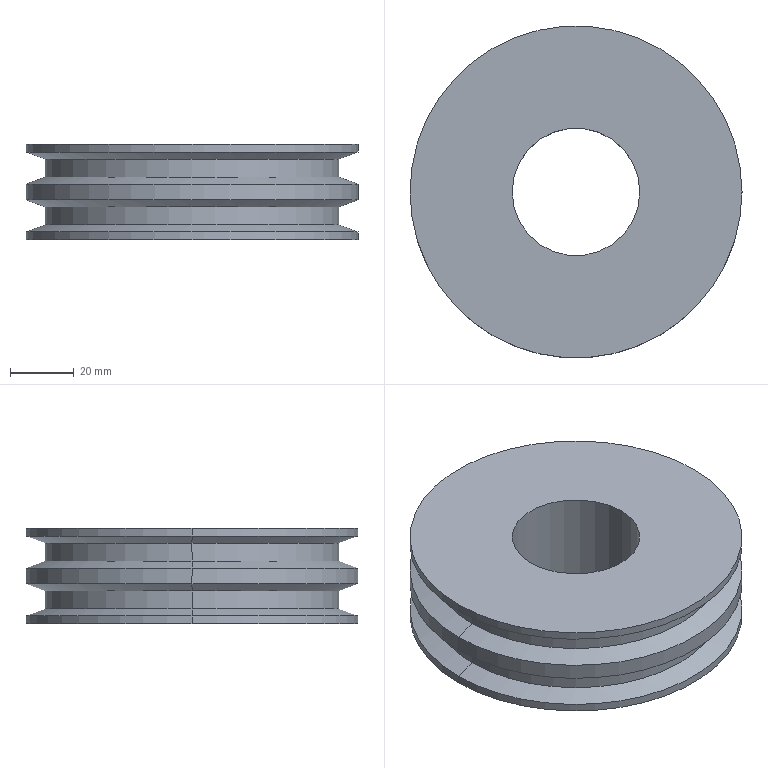Part | SolidWorks | features Extrusion 1, RevCut 1 | 1 solid | 22 faces | box 104 x 104 x 30 mm | volume 188105 mm3 | cylinder 12 | cone 8 | plane 2 | commonest cylinder face diameters 104 x6 92 x4 40 x2
STEP:
#1=CARTESIAN_POINT('',(-52.,0.,17.5));
#2=VERTEX_POINT('',#1);
#3=CARTESIAN_POINT('',(52.,0.,17.5));
#4=VERTEX_POINT('',#3);
#5=CARTESIAN_POINT('',(0.,0.,17.5));
#6=DIRECTION('',(0.,0.,-1.));
#7=DIRECTION('',(-1.,0.,0.));
#8=AXIS2_PLACEMENT_3D('',#5,#6,#7);
#9=CIRCLE('',#8,52.);
#10=EDGE_CURVE('',#2,#4,#9,.T.);
#11=ORIENTED_EDGE('',*,*,#10,.T.);
#12=CARTESIAN_POINT('',(52.,0.,12.5));
#13=VERTEX_POINT('',#12);
#14=CARTESIAN_POINT('',(52.,0.,30.));
#15=DIRECTION('',(0.,0.,-1.));
#16=VECTOR('',#15,1000.);
#17=LINE('',#14,#16);
#18=EDGE_CURVE('',#4,#13,#17,.T.);
#19=ORIENTED_EDGE('',*,*,#18,.T.);
#20=CARTESIAN_POINT('',(-52.,0.,12.5));
#21=VERTEX_POINT('',#20);
#22=CARTESIAN_POINT('',(0.,0.,12.5));
#23=DIRECTION('',(0.,0.,-1.));
#24=DIRECTION('',(-1.,0.,0.));
#25=AXIS2_PLACEMENT_3D('',#22,#23,#24);
#26=CIRCLE('',#25,52.);
#27=EDGE_CURVE('',#21,#13,#26,.T.);
#28=ORIENTED_EDGE('',*,*,#27,.F.);
#29=CARTESIAN_POINT('',(-52.,0.,30.));
#30=DIRECTION('',(0.,0.,-1.));
#31=VECTOR('',#30,1000.);
#32=LINE('',#29,#31);
#33=EDGE_CURVE('',#2,#21,#32,.T.);
#34=ORIENTED_EDGE('',*,*,#33,.F.);
#35=EDGE_LOOP('',(#11,#19,#28,#34));
#36=FACE_OUTER_BOUND('',#35,.T.);
#37=CARTESIAN_POINT('',(0.,0.,30.));
#38=DIRECTION('',(0.,0.,-1.));
#39=DIRECTION('',(-1.,0.,0.));
#40=AXIS2_PLACEMENT_3D('',#37,#38,#39);
#41=CYLINDRICAL_SURFACE('',#40,52.);
#42=ADVANCED_FACE('',(#36),#41,.T.);
#43=CARTESIAN_POINT('',(-46.,0.,19.684));
#44=VERTEX_POINT('',#43);
#45=CARTESIAN_POINT('',(46.,0.,19.684));
#46=VERTEX_POINT('',#45);
#47=CARTESIAN_POINT('',(0.,0.,19.684));
#48=DIRECTION('',(0.,0.,-1.));
#49=DIRECTION('',(-1.,0.,0.));
#50=AXIS2_PLACEMENT_3D('',#47,#48,#49);
#51=CIRCLE('',#50,46.);
#52=EDGE_CURVE('',#44,#46,#51,.T.);
#53=ORIENTED_EDGE('',*,*,#52,.T.);
#54=CARTESIAN_POINT('',(46.,0.,19.684));
#55=DIRECTION('',(0.9397,0.,-0.342));
#56=VECTOR('',#55,1000.);
#57=LINE('',#54,#56);
#58=EDGE_CURVE('',#46,#4,#57,.T.);
#59=ORIENTED_EDGE('',*,*,#58,.T.);
#60=ORIENTED_EDGE('',*,*,#10,.F.);
#61=CARTESIAN_POINT('',(-46.,0.,19.684));
#62=DIRECTION('',(-0.9397,0.,-0.342));
#63=VECTOR('',#62,1000.);
#64=LINE('',#61,#63);
#65=EDGE_CURVE('',#44,#2,#64,.T.);
#66=ORIENTED_EDGE('',*,*,#65,.F.);
#67=EDGE_LOOP('',(#53,#59,#60,#66));
#68=FACE_OUTER_BOUND('',#67,.T.);
#69=CARTESIAN_POINT('',(0.,0.,19.684));
#70=DIRECTION('',(0.,0.,-1.));
#71=DIRECTION('',(-1.,0.,0.));
#72=AXIS2_PLACEMENT_3D('',#69,#70,#71);
#73=CONICAL_SURFACE('',#72,46.,1.222);
#74=ADVANCED_FACE('',(#68),#73,.T.);
#75=CARTESIAN_POINT('',(-46.,0.,25.316));
#76=VERTEX_POINT('',#75);
#77=CARTESIAN_POINT('',(46.,0.,25.316));
#78=VERTEX_POINT('',#77);
#79=CARTESIAN_POINT('',(0.,0.,25.316));
#80=DIRECTION('',(0.,0.,-1.));
#81=DIRECTION('',(-1.,0.,0.));
#82=AXIS2_PLACEMENT_3D('',#79,#80,#81);
#83=CIRCLE('',#82,46.);
#84=EDGE_CURVE('',#76,#78,#83,.T.);
#85=ORIENTED_EDGE('',*,*,#84,.T.);
#86=CARTESIAN_POINT('',(46.,0.,0.));
#87=DIRECTION('',(0.,0.,-1.));
#88=VECTOR('',#87,1000.);
#89=LINE('',#86,#88);
#90=EDGE_CURVE('',#78,#46,#89,.T.);
#91=ORIENTED_EDGE('',*,*,#90,.T.);
#92=ORIENTED_EDGE('',*,*,#52,.F.);
#93=CARTESIAN_POINT('',(-46.,0.,0.));
#94=DIRECTION('',(0.,0.,-1.));
#95=VECTOR('',#94,1000.);
#96=LINE('',#93,#95);
#97=EDGE_CURVE('',#76,#44,#96,.T.);
#98=ORIENTED_EDGE('',*,*,#97,.F.);
#99=EDGE_LOOP('',(#85,#91,#92,#98));
#100=FACE_OUTER_BOUND('',#99,.T.);
#101=CARTESIAN_POINT('',(0.,0.,0.));
#102=DIRECTION('',(0.,0.,-1.));
#103=DIRECTION('',(-1.,0.,0.));
#104=AXIS2_PLACEMENT_3D('',#101,#102,#103);
#105=CYLINDRICAL_SURFACE('',#104,46.);
#106=ADVANCED_FACE('',(#100),#105,.T.);
#107=ORIENTED_EDGE('',*,*,#84,.F.);
#108=CARTESIAN_POINT('',(-52.,0.,27.5));
#109=VERTEX_POINT('',#108);
#110=CARTESIAN_POINT('',(-52.,0.,27.5));
#111=DIRECTION('',(-0.9397,0.,0.342));
#112=VECTOR('',#111,1000.);
#113=LINE('',#110,#112);
#114=EDGE_CURVE('',#76,#109,#113,.T.);
#115=ORIENTED_EDGE('',*,*,#114,.T.);
#116=CARTESIAN_POINT('',(52.,0.,27.5));
#117=VERTEX_POINT('',#116);
#118=CARTESIAN_POINT('',(0.,0.,27.5));
#119=DIRECTION('',(0.,0.,-1.));
#120=DIRECTION('',(-1.,0.,0.));
#121=AXIS2_PLACEMENT_3D('',#118,#119,#120);
#122=CIRCLE('',#121,52.);
#123=EDGE_CURVE('',#109,#117,#122,.T.);
#124=ORIENTED_EDGE('',*,*,#123,.T.);
#125=CARTESIAN_POINT('',(52.,0.,27.5));
#126=DIRECTION('',(0.9397,0.,0.342));
#127=VECTOR('',#126,1000.);
#128=LINE('',#125,#127);
#129=EDGE_CURVE('',#78,#117,#128,.T.);
#130=ORIENTED_EDGE('',*,*,#129,.F.);
#131=EDGE_LOOP('',(#107,#115,#124,#130));
#132=FACE_OUTER_BOUND('',#131,.T.);
#133=CARTESIAN_POINT('',(0.,0.,27.5));
#134=DIRECTION('',(0.,0.,1.));
#135=DIRECTION('',(1.,0.,0.));
#136=AXIS2_PLACEMENT_3D('',#133,#134,#135);
#137=CONICAL_SURFACE('',#136,52.,1.222);
#138=ADVANCED_FACE('',(#132),#137,.T.);
#139=CARTESIAN_POINT('',(-46.,0.,10.316));
#140=VERTEX_POINT('',#139);
#141=CARTESIAN_POINT('',(46.,0.,10.316));
#142=VERTEX_POINT('',#141);
#143=CARTESIAN_POINT('',(0.,0.,10.316));
#144=DIRECTION('',(0.,0.,-1.));
#145=DIRECTION('',(-1.,0.,0.));
#146=AXIS2_PLACEMENT_3D('',#143,#144,#145);
#147=CIRCLE('',#146,46.);
#148=EDGE_CURVE('',#140,#142,#147,.T.);
#149=ORIENTED_EDGE('',*,*,#148,.F.);
#150=CARTESIAN_POINT('',(-52.,0.,12.5));
#151=DIRECTION('',(-0.9397,0.,0.342));
#152=VECTOR('',#151,1000.);
#153=LINE('',#150,#152);
#154=EDGE_CURVE('',#140,#21,#153,.T.);
#155=ORIENTED_EDGE('',*,*,#154,.T.);
#156=ORIENTED_EDGE('',*,*,#27,.T.);
#157=CARTESIAN_POINT('',(52.,0.,12.5));
#158=DIRECTION('',(0.9397,0.,0.342));
#159=VECTOR('',#158,1000.);
#160=LINE('',#157,#159);
#161=EDGE_CURVE('',#142,#13,#160,.T.);
#162=ORIENTED_EDGE('',*,*,#161,.F.);
#163=EDGE_LOOP('',(#149,#155,#156,#162));
#164=FACE_OUTER_BOUND('',#163,.T.);
#165=CARTESIAN_POINT('',(0.,0.,12.5));
#166=DIRECTION('',(0.,0.,1.));
#167=DIRECTION('',(1.,0.,0.));
#168=AXIS2_PLACEMENT_3D('',#165,#166,#167);
#169=CONICAL_SURFACE('',#168,52.,1.222);
#170=ADVANCED_FACE('',(#164),#169,.T.);
#171=ORIENTED_EDGE('',*,*,#148,.T.);
#172=CARTESIAN_POINT('',(46.,0.,4.684));
#173=VERTEX_POINT('',#172);
#174=CARTESIAN_POINT('',(46.,0.,0.));
#175=DIRECTION('',(0.,0.,-1.));
#176=VECTOR('',#175,1000.);
#177=LINE('',#174,#176);
#178=EDGE_CURVE('',#142,#173,#177,.T.);
#179=ORIENTED_EDGE('',*,*,#178,.T.);
#180=CARTESIAN_POINT('',(-46.,0.,4.684));
#181=VERTEX_POINT('',#180);
#182=CARTESIAN_POINT('',(0.,0.,4.684));
#183=DIRECTION('',(0.,0.,-1.));
#184=DIRECTION('',(-1.,0.,0.));
#185=AXIS2_PLACEMENT_3D('',#182,#183,#184);
#186=CIRCLE('',#185,46.);
#187=EDGE_CURVE('',#181,#173,#186,.T.);
#188=ORIENTED_EDGE('',*,*,#187,.F.);
#189=CARTESIAN_POINT('',(-46.,0.,0.));
#190=DIRECTION('',(0.,0.,-1.));
#191=VECTOR('',#190,1000.);
#192=LINE('',#189,#191);
#193=EDGE_CURVE('',#140,#181,#192,.T.);
#194=ORIENTED_EDGE('',*,*,#193,.F.);
#195=EDGE_LOOP('',(#171,#179,#188,#194));
#196=FACE_OUTER_BOUND('',#195,.T.);
#197=CARTESIAN_POINT('',(0.,0.,0.));
#198=DIRECTION('',(0.,0.,-1.));
#199=DIRECTION('',(-1.,0.,0.));
#200=AXIS2_PLACEMENT_3D('',#197,#198,#199);
#201=CYLINDRICAL_SURFACE('',#200,46.);
#202=ADVANCED_FACE('',(#196),#201,.T.);
#203=ORIENTED_EDGE('',*,*,#187,.T.);
#204=CARTESIAN_POINT('',(52.,0.,2.5));
#205=VERTEX_POINT('',#204);
#206=CARTESIAN_POINT('',(46.,0.,4.684));
#207=DIRECTION('',(0.9397,0.,-0.342));
#208=VECTOR('',#207,1000.);
#209=LINE('',#206,#208);
#210=EDGE_CURVE('',#173,#205,#209,.T.);
#211=ORIENTED_EDGE('',*,*,#210,.T.);
#212=CARTESIAN_POINT('',(-52.,0.,2.5));
#213=VERTEX_POINT('',#212);
#214=CARTESIAN_POINT('',(0.,0.,2.5));
#215=DIRECTION('',(0.,0.,-1.));
#216=DIRECTION('',(-1.,0.,0.));
#217=AXIS2_PLACEMENT_3D('',#214,#215,#216);
#218=CIRCLE('',#217,52.);
#219=EDGE_CURVE('',#213,#205,#218,.T.);
#220=ORIENTED_EDGE('',*,*,#219,.F.);
#221=CARTESIAN_POINT('',(-46.,0.,4.684));
#222=DIRECTION('',(-0.9397,0.,-0.342));
#223=VECTOR('',#222,1000.);
#224=LINE('',#221,#223);
#225=EDGE_CURVE('',#181,#213,#224,.T.);
#226=ORIENTED_EDGE('',*,*,#225,.F.);
#227=EDGE_LOOP('',(#203,#211,#220,#226));
#228=FACE_OUTER_BOUND('',#227,.T.);
#229=CARTESIAN_POINT('',(0.,0.,4.684));
#230=DIRECTION('',(0.,0.,-1.));
#231=DIRECTION('',(-1.,0.,0.));
#232=AXIS2_PLACEMENT_3D('',#229,#230,#231);
#233=CONICAL_SURFACE('',#232,46.,1.222);
#234=ADVANCED_FACE('',(#228),#233,.T.);
#235=CARTESIAN_POINT('',(-20.,0.,30.));
#236=VERTEX_POINT('',#235);
#237=CARTESIAN_POINT('',(20.,0.,30.));
#238=VERTEX_POINT('',#237);
#239=CARTESIAN_POINT('',(0.,0.,30.));
#240=DIRECTION('',(0.,0.,1.));
#241=DIRECTION('',(1.,0.,0.));
#242=AXIS2_PLACEMENT_3D('',#239,#240,#241);
#243=CIRCLE('',#242,20.);
#244=EDGE_CURVE('',#236,#238,#243,.T.);
#245=ORIENTED_EDGE('',*,*,#244,.T.);
#246=CARTESIAN_POINT('',(20.,0.,0.));
#247=VERTEX_POINT('',#246);
#248=CARTESIAN_POINT('',(20.,0.,30.));
#249=DIRECTION('',(0.,0.,-1.));
#250=VECTOR('',#249,1000.);
#251=LINE('',#248,#250);
#252=EDGE_CURVE('',#238,#247,#251,.T.);
#253=ORIENTED_EDGE('',*,*,#252,.T.);
#254=CARTESIAN_POINT('',(-20.,0.,0.));
#255=VERTEX_POINT('',#254);
#256=CARTESIAN_POINT('',(0.,0.,0.));
#257=DIRECTION('',(0.,0.,1.));
#258=DIRECTION('',(1.,0.,0.));
#259=AXIS2_PLACEMENT_3D('',#256,#257,#258);
#260=CIRCLE('',#259,20.);
#261=EDGE_CURVE('',#255,#247,#260,.T.);
#262=ORIENTED_EDGE('',*,*,#261,.F.);
#263=CARTESIAN_POINT('',(-20.,0.,30.));
#264=DIRECTION('',(0.,0.,-1.));
#265=VECTOR('',#264,1000.);
#266=LINE('',#263,#265);
#267=EDGE_CURVE('',#236,#255,#266,.T.);
#268=ORIENTED_EDGE('',*,*,#267,.F.);
#269=EDGE_LOOP('',(#245,#253,#262,#268));
#270=FACE_OUTER_BOUND('',#269,.T.);
#271=CARTESIAN_POINT('',(0.,0.,30.));
#272=DIRECTION('',(0.,0.,-1.));
#273=DIRECTION('',(-1.,0.,0.));
#274=AXIS2_PLACEMENT_3D('',#271,#272,#273);
#275=CYLINDRICAL_SURFACE('',#274,20.);
#276=ADVANCED_FACE('',(#270),#275,.F.);
#277=ORIENTED_EDGE('',*,*,#219,.T.);
#278=CARTESIAN_POINT('',(52.,0.,0.));
#279=VERTEX_POINT('',#278);
#280=CARTESIAN_POINT('',(52.,0.,30.));
#281=DIRECTION('',(0.,0.,-1.));
#282=VECTOR('',#281,1000.);
#283=LINE('',#280,#282);
#284=EDGE_CURVE('',#205,#279,#283,.T.);
#285=ORIENTED_EDGE('',*,*,#284,.T.);
#286=CARTESIAN_POINT('',(-52.,0.,0.));
#287=VERTEX_POINT('',#286);
#288=CARTESIAN_POINT('',(0.,0.,0.));
#289=DIRECTION('',(0.,0.,1.));
#290=DIRECTION('',(1.,0.,0.));
#291=AXIS2_PLACEMENT_3D('',#288,#289,#290);
#292=CIRCLE('',#291,52.);
#293=EDGE_CURVE('',#279,#287,#292,.T.);
#294=ORIENTED_EDGE('',*,*,#293,.T.);
#295=CARTESIAN_POINT('',(-52.,0.,30.));
#296=DIRECTION('',(0.,0.,-1.));
#297=VECTOR('',#296,1000.);
#298=LINE('',#295,#297);
#299=EDGE_CURVE('',#213,#287,#298,.T.);
#300=ORIENTED_EDGE('',*,*,#299,.F.);
#301=EDGE_LOOP('',(#277,#285,#294,#300));
#302=FACE_OUTER_BOUND('',#301,.T.);
#303=CARTESIAN_POINT('',(0.,0.,30.));
#304=DIRECTION('',(0.,0.,-1.));
#305=DIRECTION('',(-1.,0.,0.));
#306=AXIS2_PLACEMENT_3D('',#303,#304,#305);
#307=CYLINDRICAL_SURFACE('',#306,52.);
#308=ADVANCED_FACE('',(#302),#307,.T.);
#309=CARTESIAN_POINT('',(52.,0.,30.));
#310=VERTEX_POINT('',#309);
#311=CARTESIAN_POINT('',(-52.,0.,30.));
#312=VERTEX_POINT('',#311);
#313=CARTESIAN_POINT('',(0.,0.,30.));
#314=DIRECTION('',(0.,0.,1.));
#315=DIRECTION('',(1.,0.,0.));
#316=AXIS2_PLACEMENT_3D('',#313,#314,#315);
#317=CIRCLE('',#316,52.);
#318=EDGE_CURVE('',#310,#312,#317,.T.);
#319=ORIENTED_EDGE('',*,*,#318,.F.);
#320=CARTESIAN_POINT('',(52.,0.,30.));
#321=DIRECTION('',(0.,0.,-1.));
#322=VECTOR('',#321,1000.);
#323=LINE('',#320,#322);
#324=EDGE_CURVE('',#310,#117,#323,.T.);
#325=ORIENTED_EDGE('',*,*,#324,.T.);
#326=ORIENTED_EDGE('',*,*,#123,.F.);
#327=CARTESIAN_POINT('',(-52.,0.,30.));
#328=DIRECTION('',(0.,0.,-1.));
#329=VECTOR('',#328,1000.);
#330=LINE('',#327,#329);
#331=EDGE_CURVE('',#312,#109,#330,.T.);
#332=ORIENTED_EDGE('',*,*,#331,.F.);
#333=EDGE_LOOP('',(#319,#325,#326,#332));
#334=FACE_OUTER_BOUND('',#333,.T.);
#335=CARTESIAN_POINT('',(0.,0.,30.));
#336=DIRECTION('',(0.,0.,-1.));
#337=DIRECTION('',(-1.,0.,0.));
#338=AXIS2_PLACEMENT_3D('',#335,#336,#337);
#339=CYLINDRICAL_SURFACE('',#338,52.);
#340=ADVANCED_FACE('',(#334),#339,.T.);
#341=ORIENTED_EDGE('',*,*,#324,.F.);
#342=CARTESIAN_POINT('',(0.,0.,30.));
#343=DIRECTION('',(0.,0.,1.));
#344=DIRECTION('',(1.,0.,0.));
#345=AXIS2_PLACEMENT_3D('',#342,#343,#344);
#346=CIRCLE('',#345,52.);
#347=EDGE_CURVE('',#312,#310,#346,.T.);
#348=ORIENTED_EDGE('',*,*,#347,.F.);
#349=ORIENTED_EDGE('',*,*,#331,.T.);
#350=CARTESIAN_POINT('',(0.,0.,27.5));
#351=DIRECTION('',(0.,0.,-1.));
#352=DIRECTION('',(-1.,0.,0.));
#353=AXIS2_PLACEMENT_3D('',#350,#351,#352);
#354=CIRCLE('',#353,52.);
#355=EDGE_CURVE('',#117,#109,#354,.T.);
#356=ORIENTED_EDGE('',*,*,#355,.F.);
#357=EDGE_LOOP('',(#341,#348,#349,#356));
#358=FACE_OUTER_BOUND('',#357,.T.);
#359=CARTESIAN_POINT('',(0.,0.,30.));
#360=DIRECTION('',(0.,0.,-1.));
#361=DIRECTION('',(-1.,0.,0.));
#362=AXIS2_PLACEMENT_3D('',#359,#360,#361);
#363=CYLINDRICAL_SURFACE('',#362,52.);
#364=ADVANCED_FACE('',(#358),#363,.T.);
#365=ORIENTED_EDGE('',*,*,#284,.F.);
#366=CARTESIAN_POINT('',(0.,0.,2.5));
#367=DIRECTION('',(0.,0.,-1.));
#368=DIRECTION('',(-1.,0.,0.));
#369=AXIS2_PLACEMENT_3D('',#366,#367,#368);
#370=CIRCLE('',#369,52.);
#371=EDGE_CURVE('',#205,#213,#370,.T.);
#372=ORIENTED_EDGE('',*,*,#371,.T.);
#373=ORIENTED_EDGE('',*,*,#299,.T.);
#374=CARTESIAN_POINT('',(0.,0.,0.));
#375=DIRECTION('',(0.,0.,1.));
#376=DIRECTION('',(1.,0.,0.));
#377=AXIS2_PLACEMENT_3D('',#374,#375,#376);
#378=CIRCLE('',#377,52.);
#379=EDGE_CURVE('',#287,#279,#378,.T.);
#380=ORIENTED_EDGE('',*,*,#379,.T.);
#381=EDGE_LOOP('',(#365,#372,#373,#380));
#382=FACE_OUTER_BOUND('',#381,.T.);
#383=CARTESIAN_POINT('',(0.,0.,30.));
#384=DIRECTION('',(0.,0.,-1.));
#385=DIRECTION('',(-1.,0.,0.));
#386=AXIS2_PLACEMENT_3D('',#383,#384,#385);
#387=CYLINDRICAL_SURFACE('',#386,52.);
#388=ADVANCED_FACE('',(#382),#387,.T.);
#389=ORIENTED_EDGE('',*,*,#347,.T.);
#390=ORIENTED_EDGE('',*,*,#318,.T.);
#391=EDGE_LOOP('',(#389,#390));
#392=FACE_OUTER_BOUND('',#391,.T.);
#393=ORIENTED_EDGE('',*,*,#244,.F.);
#394=CARTESIAN_POINT('',(0.,0.,30.));
#395=DIRECTION('',(0.,0.,1.));
#396=DIRECTION('',(1.,0.,0.));
#397=AXIS2_PLACEMENT_3D('',#394,#395,#396);
#398=CIRCLE('',#397,20.);
#399=EDGE_CURVE('',#238,#236,#398,.T.);
#400=ORIENTED_EDGE('',*,*,#399,.F.);
#401=EDGE_LOOP('',(#393,#400));
#402=FACE_BOUND('',#401,.T.);
#403=CARTESIAN_POINT('',(0.,0.,30.));
#404=DIRECTION('',(0.,0.,1.));
#405=DIRECTION('',(1.,0.,0.));
#406=AXIS2_PLACEMENT_3D('',#403,#404,#405);
#407=PLANE('',#406);
#408=ADVANCED_FACE('',(#392,#402),#407,.T.);
#409=ORIENTED_EDGE('',*,*,#379,.F.);
#410=ORIENTED_EDGE('',*,*,#293,.F.);
#411=EDGE_LOOP('',(#409,#410));
#412=FACE_OUTER_BOUND('',#411,.T.);
#413=ORIENTED_EDGE('',*,*,#261,.T.);
#414=CARTESIAN_POINT('',(0.,0.,0.));
#415=DIRECTION('',(0.,0.,1.));
#416=DIRECTION('',(1.,0.,0.));
#417=AXIS2_PLACEMENT_3D('',#414,#415,#416);
#418=CIRCLE('',#417,20.);
#419=EDGE_CURVE('',#247,#255,#418,.T.);
#420=ORIENTED_EDGE('',*,*,#419,.T.);
#421=EDGE_LOOP('',(#413,#420));
#422=FACE_BOUND('',#421,.T.);
#423=CARTESIAN_POINT('',(0.,0.,0.));
#424=DIRECTION('',(0.,0.,1.));
#425=DIRECTION('',(1.,0.,0.));
#426=AXIS2_PLACEMENT_3D('',#423,#424,#425);
#427=PLANE('',#426);
#428=ADVANCED_FACE('',(#412,#422),#427,.F.);
#429=ORIENTED_EDGE('',*,*,#252,.F.);
#430=ORIENTED_EDGE('',*,*,#399,.T.);
#431=ORIENTED_EDGE('',*,*,#267,.T.);
#432=ORIENTED_EDGE('',*,*,#419,.F.);
#433=EDGE_LOOP('',(#429,#430,#431,#432));
#434=FACE_OUTER_BOUND('',#433,.T.);
#435=CARTESIAN_POINT('',(0.,0.,30.));
#436=DIRECTION('',(0.,0.,-1.));
#437=DIRECTION('',(-1.,0.,0.));
#438=AXIS2_PLACEMENT_3D('',#435,#436,#437);
#439=CYLINDRICAL_SURFACE('',#438,20.);
#440=ADVANCED_FACE('',(#434),#439,.F.);
#441=ORIENTED_EDGE('',*,*,#210,.F.);
#442=CARTESIAN_POINT('',(0.,0.,4.684));
#443=DIRECTION('',(0.,0.,-1.));
#444=DIRECTION('',(-1.,0.,0.));
#445=AXIS2_PLACEMENT_3D('',#442,#443,#444);
#446=CIRCLE('',#445,46.);
#447=EDGE_CURVE('',#173,#181,#446,.T.);
#448=ORIENTED_EDGE('',*,*,#447,.T.);
#449=ORIENTED_EDGE('',*,*,#225,.T.);
#450=ORIENTED_EDGE('',*,*,#371,.F.);
#451=EDGE_LOOP('',(#441,#448,#449,#450));
#452=FACE_OUTER_BOUND('',#451,.T.);
#453=CARTESIAN_POINT('',(0.,0.,4.684));
#454=DIRECTION('',(0.,0.,-1.));
#455=DIRECTION('',(-1.,0.,0.));
#456=AXIS2_PLACEMENT_3D('',#453,#454,#455);
#457=CONICAL_SURFACE('',#456,46.,1.222);
#458=ADVANCED_FACE('',(#452),#457,.T.);
#459=ORIENTED_EDGE('',*,*,#178,.F.);
#460=CARTESIAN_POINT('',(0.,0.,10.316));
#461=DIRECTION('',(0.,0.,-1.));
#462=DIRECTION('',(-1.,0.,0.));
#463=AXIS2_PLACEMENT_3D('',#460,#461,#462);
#464=CIRCLE('',#463,46.);
#465=EDGE_CURVE('',#142,#140,#464,.T.);
#466=ORIENTED_EDGE('',*,*,#465,.T.);
#467=ORIENTED_EDGE('',*,*,#193,.T.);
#468=ORIENTED_EDGE('',*,*,#447,.F.);
#469=EDGE_LOOP('',(#459,#466,#467,#468));
#470=FACE_OUTER_BOUND('',#469,.T.);
#471=CARTESIAN_POINT('',(0.,0.,0.));
#472=DIRECTION('',(0.,0.,-1.));
#473=DIRECTION('',(-1.,0.,0.));
#474=AXIS2_PLACEMENT_3D('',#471,#472,#473);
#475=CYLINDRICAL_SURFACE('',#474,46.);
#476=ADVANCED_FACE('',(#470),#475,.T.);
#477=ORIENTED_EDGE('',*,*,#154,.F.);
#478=ORIENTED_EDGE('',*,*,#465,.F.);
#479=ORIENTED_EDGE('',*,*,#161,.T.);
#480=CARTESIAN_POINT('',(0.,0.,12.5));
#481=DIRECTION('',(0.,0.,-1.));
#482=DIRECTION('',(-1.,0.,0.));
#483=AXIS2_PLACEMENT_3D('',#480,#481,#482);
#484=CIRCLE('',#483,52.);
#485=EDGE_CURVE('',#13,#21,#484,.T.);
#486=ORIENTED_EDGE('',*,*,#485,.T.);
#487=EDGE_LOOP('',(#477,#478,#479,#486));
#488=FACE_OUTER_BOUND('',#487,.T.);
#489=CARTESIAN_POINT('',(0.,0.,12.5));
#490=DIRECTION('',(0.,0.,1.));
#491=DIRECTION('',(1.,0.,0.));
#492=AXIS2_PLACEMENT_3D('',#489,#490,#491);
#493=CONICAL_SURFACE('',#492,52.,1.222);
#494=ADVANCED_FACE('',(#488),#493,.T.);
#495=ORIENTED_EDGE('',*,*,#114,.F.);
#496=CARTESIAN_POINT('',(0.,0.,25.316));
#497=DIRECTION('',(0.,0.,-1.));
#498=DIRECTION('',(-1.,0.,0.));
#499=AXIS2_PLACEMENT_3D('',#496,#497,#498);
#500=CIRCLE('',#499,46.);
#501=EDGE_CURVE('',#78,#76,#500,.T.);
#502=ORIENTED_EDGE('',*,*,#501,.F.);
#503=ORIENTED_EDGE('',*,*,#129,.T.);
#504=ORIENTED_EDGE('',*,*,#355,.T.);
#505=EDGE_LOOP('',(#495,#502,#503,#504));
#506=FACE_OUTER_BOUND('',#505,.T.);
#507=CARTESIAN_POINT('',(0.,0.,27.5));
#508=DIRECTION('',(0.,0.,1.));
#509=DIRECTION('',(1.,0.,0.));
#510=AXIS2_PLACEMENT_3D('',#507,#508,#509);
#511=CONICAL_SURFACE('',#510,52.,1.222);
#512=ADVANCED_FACE('',(#506),#511,.T.);
#513=ORIENTED_EDGE('',*,*,#90,.F.);
#514=ORIENTED_EDGE('',*,*,#501,.T.);
#515=ORIENTED_EDGE('',*,*,#97,.T.);
#516=CARTESIAN_POINT('',(0.,0.,19.684));
#517=DIRECTION('',(0.,0.,-1.));
#518=DIRECTION('',(-1.,0.,0.));
#519=AXIS2_PLACEMENT_3D('',#516,#517,#518);
#520=CIRCLE('',#519,46.);
#521=EDGE_CURVE('',#46,#44,#520,.T.);
#522=ORIENTED_EDGE('',*,*,#521,.F.);
#523=EDGE_LOOP('',(#513,#514,#515,#522));
#524=FACE_OUTER_BOUND('',#523,.T.);
#525=CARTESIAN_POINT('',(0.,0.,0.));
#526=DIRECTION('',(0.,0.,-1.));
#527=DIRECTION('',(-1.,0.,0.));
#528=AXIS2_PLACEMENT_3D('',#525,#526,#527);
#529=CYLINDRICAL_SURFACE('',#528,46.);
#530=ADVANCED_FACE('',(#524),#529,.T.);
#531=ORIENTED_EDGE('',*,*,#58,.F.);
#532=ORIENTED_EDGE('',*,*,#521,.T.);
#533=ORIENTED_EDGE('',*,*,#65,.T.);
#534=CARTESIAN_POINT('',(0.,0.,17.5));
#535=DIRECTION('',(0.,0.,-1.));
#536=DIRECTION('',(-1.,0.,0.));
#537=AXIS2_PLACEMENT_3D('',#534,#535,#536);
#538=CIRCLE('',#537,52.);
#539=EDGE_CURVE('',#4,#2,#538,.T.);
#540=ORIENTED_EDGE('',*,*,#539,.F.);
#541=EDGE_LOOP('',(#531,#532,#533,#540));
#542=FACE_OUTER_BOUND('',#541,.T.);
#543=CARTESIAN_POINT('',(0.,0.,19.684));
#544=DIRECTION('',(0.,0.,-1.));
#545=DIRECTION('',(-1.,0.,0.));
#546=AXIS2_PLACEMENT_3D('',#543,#544,#545);
#547=CONICAL_SURFACE('',#546,46.,1.222);
#548=ADVANCED_FACE('',(#542),#547,.T.);
#549=ORIENTED_EDGE('',*,*,#18,.F.);
#550=ORIENTED_EDGE('',*,*,#539,.T.);
#551=ORIENTED_EDGE('',*,*,#33,.T.);
#552=ORIENTED_EDGE('',*,*,#485,.F.);
#553=EDGE_LOOP('',(#549,#550,#551,#552));
#554=FACE_OUTER_BOUND('',#553,.T.);
#555=CARTESIAN_POINT('',(0.,0.,30.));
#556=DIRECTION('',(0.,0.,-1.));
#557=DIRECTION('',(-1.,0.,0.));
#558=AXIS2_PLACEMENT_3D('',#555,#556,#557);
#559=CYLINDRICAL_SURFACE('',#558,52.);
#560=ADVANCED_FACE('',(#554),#559,.T.);
#561=CLOSED_SHELL('',(#42,#74,#106,#138,#170,#202,#234,#276,#308,#340,#364,#388,#408,#428,#440,#458,#476,#494,#512,#530,#548,#560));
#562=MANIFOLD_SOLID_BREP('',#561);
#563=CARTESIAN_POINT('',(0.,0.,0.));
#564=DIRECTION('',(0.,0.,1.));
#565=DIRECTION('',(1.,0.,0.));
#566=AXIS2_PLACEMENT_3D('',#563,#564,#565);
#567=(LENGTH_UNIT()NAMED_UNIT(*)SI_UNIT(.MILLI.,.METRE.));
#568=UNCERTAINTY_MEASURE_WITH_UNIT(LENGTH_MEASURE(0.00001),#567,'','');
#569=(NAMED_UNIT(*)PLANE_ANGLE_UNIT()SI_UNIT($,.RADIAN.));
#570=(NAMED_UNIT(*)SI_UNIT($,.STERADIAN.)SOLID_ANGLE_UNIT());
#571=(GEOMETRIC_REPRESENTATION_CONTEXT(3)GLOBAL_UNCERTAINTY_ASSIGNED_CONTEXT((#568))GLOBAL_UNIT_ASSIGNED_CONTEXT((#567,#569,#570))REPRESENTATION_CONTEXT('',''));
#572=ADVANCED_BREP_SHAPE_REPRESENTATION('',(#562,#566),#571);